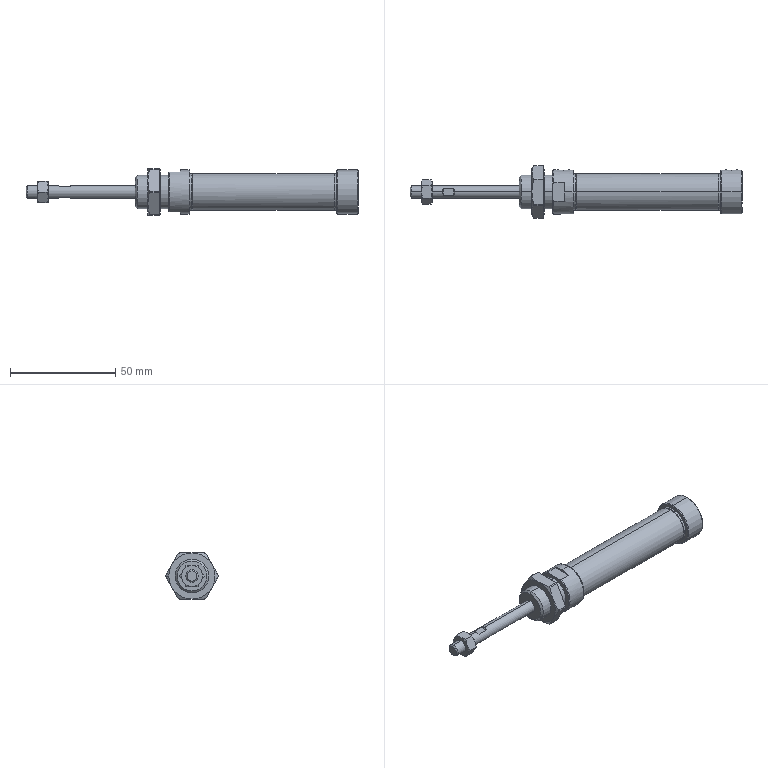Part | SolidWorks | features BaseBody 4, MoveFace 2 | 4 solids | 124 faces | box 158 x 25 x 22 mm | volume 25129 mm3 | plane 41 | cone 39 | cylinder 36 | spline 8 | commonest cylinder face diameters 17.4 x6 25 x6 4.134 x4 6 x4 16 x4 21 x4